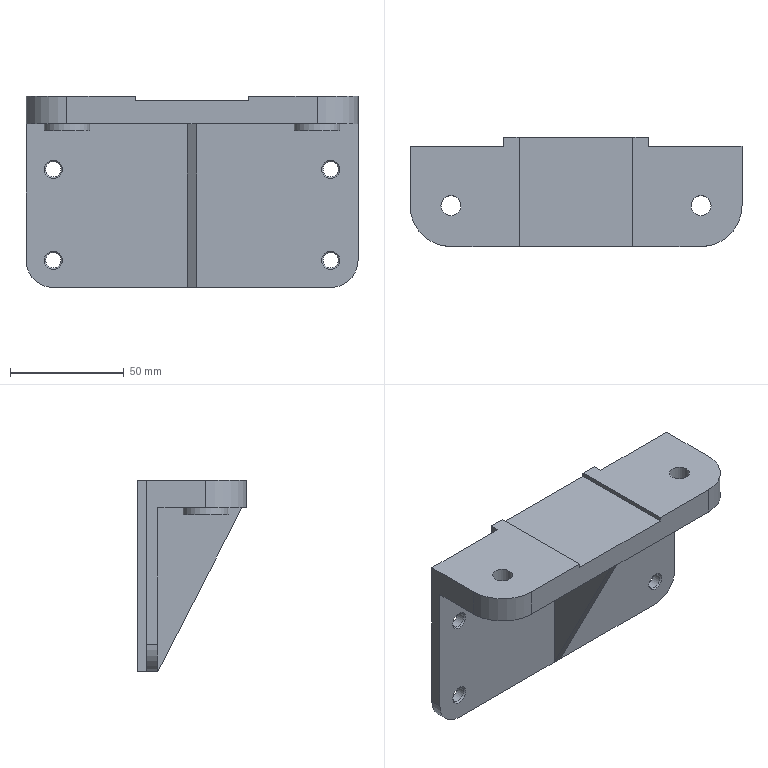Part | NX | features DATUM_CSYS 6, SIMPLE HOLE 6, SKETCH 5, SYMBOLIC_THREAD 4, EXTRUDE 3, CYLINDER 2, HOLE PACKAGE 2, BLEND 1, CPROJ 1, Intersection Curve 1, RIB 1 | 1 solid | 42 faces | box 146 x 48 x 84 mm | volume 149346 mm3 | plane 22 | cylinder 12 | cone 8 | commonest cylinder face diameters 6.8 x4 8.8 x2 20 x2 24 x2 36 x2
STEP:
#1=CARTESIAN_POINT('',(61.,37.,-16.));
#2=VERTEX_POINT('',#1);
#3=CARTESIAN_POINT('',(61.,37.,-20.));
#4=DIRECTION('',(0.,1.,0.));
#5=DIRECTION('',(0.,0.,1.));
#6=AXIS2_PLACEMENT_3D('',#3,#4,#5);
#7=CIRCLE('',#6,4.);
#8=EDGE_CURVE('',#2,#2,#7,.T.);
#9=ORIENTED_EDGE('',*,*,#8,.T.);
#10=EDGE_LOOP('',(#9));
#11=FACE_BOUND('',#10,.T.);
#12=CARTESIAN_POINT('',(61.,37.,-56.));
#13=VERTEX_POINT('',#12);
#14=CARTESIAN_POINT('',(61.,37.,-60.));
#15=DIRECTION('',(0.,1.,0.));
#16=DIRECTION('',(0.,0.,1.));
#17=AXIS2_PLACEMENT_3D('',#14,#15,#16);
#18=CIRCLE('',#17,4.);
#19=EDGE_CURVE('',#13,#13,#18,.T.);
#20=ORIENTED_EDGE('',*,*,#19,.T.);
#21=EDGE_LOOP('',(#20));
#22=FACE_BOUND('',#21,.T.);
#23=CARTESIAN_POINT('',(73.,37.,0.));
#24=VERTEX_POINT('',#23);
#25=CARTESIAN_POINT('',(2.,37.,0.));
#26=VERTEX_POINT('',#25);
#27=CARTESIAN_POINT('',(-55.,37.,0.));
#28=DIRECTION('',(-1.,0.,0.));
#29=VECTOR('',#28,1000.);
#30=LINE('',#27,#29);
#31=EDGE_CURVE('',#24,#26,#30,.T.);
#32=ORIENTED_EDGE('',*,*,#31,.T.);
#33=CARTESIAN_POINT('',(2.,37.,-72.));
#34=VERTEX_POINT('',#33);
#35=CARTESIAN_POINT('',(2.,37.,0.));
#36=DIRECTION('',(0.,0.,-1.));
#37=VECTOR('',#36,1000.);
#38=LINE('',#35,#37);
#39=EDGE_CURVE('',#26,#34,#38,.T.);
#40=ORIENTED_EDGE('',*,*,#39,.T.);
#41=CARTESIAN_POINT('',(61.,37.,-72.));
#42=VERTEX_POINT('',#41);
#43=CARTESIAN_POINT('',(73.,37.,-72.));
#44=DIRECTION('',(-1.,0.,0.));
#45=VECTOR('',#44,1000.);
#46=LINE('',#43,#45);
#47=EDGE_CURVE('',#42,#34,#46,.T.);
#48=ORIENTED_EDGE('',*,*,#47,.F.);
#49=CARTESIAN_POINT('',(73.,37.,-60.));
#50=VERTEX_POINT('',#49);
#51=CARTESIAN_POINT('',(61.,37.,-60.));
#52=DIRECTION('',(0.,1.,0.));
#53=DIRECTION('',(0.,0.,1.));
#54=AXIS2_PLACEMENT_3D('',#51,#52,#53);
#55=CIRCLE('',#54,12.);
#56=EDGE_CURVE('',#42,#50,#55,.F.);
#57=ORIENTED_EDGE('',*,*,#56,.T.);
#58=CARTESIAN_POINT('',(73.,37.,-72.));
#59=DIRECTION('',(0.,0.,1.));
#60=VECTOR('',#59,1000.);
#61=LINE('',#58,#60);
#62=EDGE_CURVE('',#50,#24,#61,.T.);
#63=ORIENTED_EDGE('',*,*,#62,.T.);
#64=EDGE_LOOP('',(#32,#40,#48,#57,#63));
#65=FACE_BOUND('',#64,.T.);
#66=CARTESIAN_POINT('',(73.,37.,-72.));
#67=DIRECTION('',(0.,1.,0.));
#68=DIRECTION('',(0.,0.,1.));
#69=AXIS2_PLACEMENT_3D('',#66,#67,#68);
#70=PLANE('',#69);
#71=ADVANCED_FACE('',(#11,#22,#65),#70,.F.);
#72=CARTESIAN_POINT('',(-50.6,16.,12.));
#73=VERTEX_POINT('',#72);
#74=CARTESIAN_POINT('',(-55.,16.,12.));
#75=DIRECTION('',(0.,0.,1.));
#76=DIRECTION('',(1.,0.,0.));
#77=AXIS2_PLACEMENT_3D('',#74,#75,#76);
#78=CIRCLE('',#77,4.4);
#79=EDGE_CURVE('',#73,#73,#78,.T.);
#80=ORIENTED_EDGE('',*,*,#79,.F.);
#81=EDGE_LOOP('',(#80));
#82=FACE_BOUND('',#81,.T.);
#83=CARTESIAN_POINT('',(-55.,-2.,12.));
#84=VERTEX_POINT('',#83);
#85=CARTESIAN_POINT('',(-25.,-2.,12.));
#86=VERTEX_POINT('',#85);
#87=CARTESIAN_POINT('',(-55.,-2.,12.));
#88=DIRECTION('',(1.,0.,0.));
#89=VECTOR('',#88,1000.);
#90=LINE('',#87,#89);
#91=EDGE_CURVE('',#84,#86,#90,.T.);
#92=ORIENTED_EDGE('',*,*,#91,.T.);
#93=CARTESIAN_POINT('',(-25.,46.,12.));
#94=VERTEX_POINT('',#93);
#95=CARTESIAN_POINT('',(-25.,-50.,12.));
#96=DIRECTION('',(0.,1.,0.));
#97=VECTOR('',#96,1000.);
#98=LINE('',#95,#97);
#99=EDGE_CURVE('',#86,#94,#98,.T.);
#100=ORIENTED_EDGE('',*,*,#99,.T.);
#101=CARTESIAN_POINT('',(-32.,46.,12.));
#102=VERTEX_POINT('',#101);
#103=CARTESIAN_POINT('',(32.,46.,12.));
#104=DIRECTION('',(-1.,0.,0.));
#105=VECTOR('',#104,1000.);
#106=LINE('',#103,#105);
#107=EDGE_CURVE('',#94,#102,#106,.T.);
#108=ORIENTED_EDGE('',*,*,#107,.T.);
#109=CARTESIAN_POINT('',(-32.,42.,12.));
#110=VERTEX_POINT('',#109);
#111=CARTESIAN_POINT('',(-32.,46.,12.));
#112=DIRECTION('',(0.,-1.,0.));
#113=VECTOR('',#112,1000.);
#114=LINE('',#111,#113);
#115=EDGE_CURVE('',#102,#110,#114,.T.);
#116=ORIENTED_EDGE('',*,*,#115,.T.);
#117=CARTESIAN_POINT('',(-73.,42.,12.));
#118=VERTEX_POINT('',#117);
#119=CARTESIAN_POINT('',(73.,42.,12.));
#120=DIRECTION('',(-1.,0.,0.));
#121=VECTOR('',#120,1000.);
#122=LINE('',#119,#121);
#123=EDGE_CURVE('',#110,#118,#122,.T.);
#124=ORIENTED_EDGE('',*,*,#123,.T.);
#125=CARTESIAN_POINT('',(-73.,16.,12.));
#126=VERTEX_POINT('',#125);
#127=CARTESIAN_POINT('',(-73.,42.,12.));
#128=DIRECTION('',(0.,-1.,0.));
#129=VECTOR('',#128,1000.);
#130=LINE('',#127,#129);
#131=EDGE_CURVE('',#118,#126,#130,.T.);
#132=ORIENTED_EDGE('',*,*,#131,.T.);
#133=CARTESIAN_POINT('',(-55.,16.,12.));
#134=DIRECTION('',(0.,0.,1.));
#135=DIRECTION('',(1.,0.,0.));
#136=AXIS2_PLACEMENT_3D('',#133,#134,#135);
#137=CIRCLE('',#136,18.);
#138=EDGE_CURVE('',#126,#84,#137,.T.);
#139=ORIENTED_EDGE('',*,*,#138,.T.);
#140=EDGE_LOOP('',(#92,#100,#108,#116,#124,#132,#139));
#141=FACE_BOUND('',#140,.T.);
#142=CARTESIAN_POINT('',(-55.,16.,12.));
#143=DIRECTION('',(0.,0.,1.));
#144=DIRECTION('',(1.,0.,0.));
#145=AXIS2_PLACEMENT_3D('',#142,#143,#144);
#146=PLANE('',#145);
#147=ADVANCED_FACE('',(#82,#141),#146,.T.);
#148=CARTESIAN_POINT('',(-61.,42.,-64.));
#149=VERTEX_POINT('',#148);
#150=CARTESIAN_POINT('',(-61.,42.,-60.));
#151=DIRECTION('',(0.,-1.,0.));
#152=DIRECTION('',(0.,0.,-1.));
#153=AXIS2_PLACEMENT_3D('',#150,#151,#152);
#154=CIRCLE('',#153,4.);
#155=EDGE_CURVE('',#149,#149,#154,.T.);
#156=ORIENTED_EDGE('',*,*,#155,.T.);
#157=EDGE_LOOP('',(#156));
#158=FACE_BOUND('',#157,.T.);
#159=CARTESIAN_POINT('',(-61.,42.,-24.));
#160=VERTEX_POINT('',#159);
#161=CARTESIAN_POINT('',(-61.,42.,-20.));
#162=DIRECTION('',(0.,-1.,0.));
#163=DIRECTION('',(0.,0.,-1.));
#164=AXIS2_PLACEMENT_3D('',#161,#162,#163);
#165=CIRCLE('',#164,4.);
#166=EDGE_CURVE('',#160,#160,#165,.T.);
#167=ORIENTED_EDGE('',*,*,#166,.T.);
#168=EDGE_LOOP('',(#167));
#169=FACE_BOUND('',#168,.T.);
#170=CARTESIAN_POINT('',(-61.,42.,-72.));
#171=VERTEX_POINT('',#170);
#172=CARTESIAN_POINT('',(-32.,42.,-72.));
#173=VERTEX_POINT('',#172);
#174=CARTESIAN_POINT('',(-73.,42.,-72.));
#175=DIRECTION('',(1.,0.,0.));
#176=VECTOR('',#175,1000.);
#177=LINE('',#174,#176);
#178=EDGE_CURVE('',#171,#173,#177,.T.);
#179=ORIENTED_EDGE('',*,*,#178,.F.);
#180=CARTESIAN_POINT('',(-73.,42.,-60.));
#181=VERTEX_POINT('',#180);
#182=CARTESIAN_POINT('',(-61.,42.,-60.));
#183=DIRECTION('',(0.,-1.,0.));
#184=DIRECTION('',(0.,0.,-1.));
#185=AXIS2_PLACEMENT_3D('',#182,#183,#184);
#186=CIRCLE('',#185,12.);
#187=EDGE_CURVE('',#171,#181,#186,.F.);
#188=ORIENTED_EDGE('',*,*,#187,.T.);
#189=CARTESIAN_POINT('',(-73.,42.,12.));
#190=DIRECTION('',(0.,0.,-1.));
#191=VECTOR('',#190,1000.);
#192=LINE('',#189,#191);
#193=EDGE_CURVE('',#118,#181,#192,.T.);
#194=ORIENTED_EDGE('',*,*,#193,.F.);
#195=ORIENTED_EDGE('',*,*,#123,.F.);
#196=CARTESIAN_POINT('',(-32.,42.,-72.));
#197=DIRECTION('',(0.,0.,1.));
#198=VECTOR('',#197,1000.);
#199=LINE('',#196,#198);
#200=EDGE_CURVE('',#173,#110,#199,.T.);
#201=ORIENTED_EDGE('',*,*,#200,.F.);
#202=EDGE_LOOP('',(#179,#188,#194,#195,#201));
#203=FACE_BOUND('',#202,.T.);
#204=CARTESIAN_POINT('',(73.,42.,12.));
#205=DIRECTION('',(0.,-1.,0.));
#206=DIRECTION('',(0.,0.,-1.));
#207=AXIS2_PLACEMENT_3D('',#204,#205,#206);
#208=PLANE('',#207);
#209=ADVANCED_FACE('',(#158,#169,#203),#208,.F.);
#210=CARTESIAN_POINT('',(-45.,16.,0.));
#211=VERTEX_POINT('',#210);
#212=CARTESIAN_POINT('',(-55.,16.,0.));
#213=DIRECTION('',(0.,0.,-1.));
#214=DIRECTION('',(1.,0.,0.));
#215=AXIS2_PLACEMENT_3D('',#212,#213,#214);
#216=CIRCLE('',#215,10.);
#217=EDGE_CURVE('',#211,#211,#216,.T.);
#218=ORIENTED_EDGE('',*,*,#217,.F.);
#219=EDGE_LOOP('',(#218));
#220=FACE_BOUND('',#219,.T.);
#221=CARTESIAN_POINT('',(65.,16.,0.));
#222=VERTEX_POINT('',#221);
#223=CARTESIAN_POINT('',(55.,16.,0.));
#224=DIRECTION('',(0.,0.,-1.));
#225=DIRECTION('',(1.,0.,0.));
#226=AXIS2_PLACEMENT_3D('',#223,#224,#225);
#227=CIRCLE('',#226,10.);
#228=EDGE_CURVE('',#222,#222,#227,.T.);
#229=ORIENTED_EDGE('',*,*,#228,.F.);
#230=EDGE_LOOP('',(#229));
#231=FACE_BOUND('',#230,.T.);
#232=CARTESIAN_POINT('',(-2.,0.,0.));
#233=VERTEX_POINT('',#232);
#234=CARTESIAN_POINT('',(2.,0.,0.));
#235=VERTEX_POINT('',#234);
#236=CARTESIAN_POINT('',(2.,0.,0.));
#237=DIRECTION('',(-1.,0.,0.));
#238=VECTOR('',#237,1000.);
#239=LINE('',#236,#238);
#240=EDGE_CURVE('',#233,#235,#239,.F.);
#241=ORIENTED_EDGE('',*,*,#240,.T.);
#242=CARTESIAN_POINT('',(2.,0.,0.));
#243=DIRECTION('',(0.,1.,0.));
#244=VECTOR('',#243,1000.);
#245=LINE('',#242,#244);
#246=EDGE_CURVE('',#235,#26,#245,.T.);
#247=ORIENTED_EDGE('',*,*,#246,.T.);
#248=ORIENTED_EDGE('',*,*,#31,.F.);
#249=CARTESIAN_POINT('',(73.,16.,0.));
#250=VERTEX_POINT('',#249);
#251=CARTESIAN_POINT('',(73.,16.,0.));
#252=DIRECTION('',(0.,1.,0.));
#253=VECTOR('',#252,1000.);
#254=LINE('',#251,#253);
#255=EDGE_CURVE('',#250,#24,#254,.T.);
#256=ORIENTED_EDGE('',*,*,#255,.F.);
#257=CARTESIAN_POINT('',(55.,-2.,0.));
#258=VERTEX_POINT('',#257);
#259=CARTESIAN_POINT('',(55.,16.,0.));
#260=DIRECTION('',(0.,0.,1.));
#261=DIRECTION('',(1.,0.,0.));
#262=AXIS2_PLACEMENT_3D('',#259,#260,#261);
#263=CIRCLE('',#262,18.);
#264=EDGE_CURVE('',#258,#250,#263,.T.);
#265=ORIENTED_EDGE('',*,*,#264,.F.);
#266=CARTESIAN_POINT('',(-55.,-2.,0.));
#267=VERTEX_POINT('',#266);
#268=CARTESIAN_POINT('',(-55.,-2.,0.));
#269=DIRECTION('',(1.,0.,0.));
#270=VECTOR('',#269,1000.);
#271=LINE('',#268,#270);
#272=EDGE_CURVE('',#267,#258,#271,.T.);
#273=ORIENTED_EDGE('',*,*,#272,.F.);
#274=CARTESIAN_POINT('',(-73.,16.,0.));
#275=VERTEX_POINT('',#274);
#276=CARTESIAN_POINT('',(-55.,16.,0.));
#277=DIRECTION('',(0.,0.,1.));
#278=DIRECTION('',(1.,0.,0.));
#279=AXIS2_PLACEMENT_3D('',#276,#277,#278);
#280=CIRCLE('',#279,18.);
#281=EDGE_CURVE('',#275,#267,#280,.T.);
#282=ORIENTED_EDGE('',*,*,#281,.F.);
#283=CARTESIAN_POINT('',(-73.,37.,0.));
#284=VERTEX_POINT('',#283);
#285=CARTESIAN_POINT('',(-73.,42.,0.));
#286=DIRECTION('',(0.,-1.,0.));
#287=VECTOR('',#286,1000.);
#288=LINE('',#285,#287);
#289=EDGE_CURVE('',#284,#275,#288,.T.);
#290=ORIENTED_EDGE('',*,*,#289,.F.);
#291=CARTESIAN_POINT('',(-2.,37.,0.));
#292=VERTEX_POINT('',#291);
#293=CARTESIAN_POINT('',(-55.,37.,0.));
#294=DIRECTION('',(-1.,0.,0.));
#295=VECTOR('',#294,1000.);
#296=LINE('',#293,#295);
#297=EDGE_CURVE('',#292,#284,#296,.T.);
#298=ORIENTED_EDGE('',*,*,#297,.F.);
#299=CARTESIAN_POINT('',(-2.,0.,0.));
#300=DIRECTION('',(0.,1.,0.));
#301=VECTOR('',#300,1000.);
#302=LINE('',#299,#301);
#303=EDGE_CURVE('',#292,#233,#302,.F.);
#304=ORIENTED_EDGE('',*,*,#303,.T.);
#305=EDGE_LOOP('',(#241,#247,#248,#256,#265,#273,#282,#290,#298,#304));
#306=FACE_BOUND('',#305,.T.);
#307=CARTESIAN_POINT('',(-55.,16.,0.));
#308=DIRECTION('',(0.,0.,1.));
#309=DIRECTION('',(1.,0.,0.));
#310=AXIS2_PLACEMENT_3D('',#307,#308,#309);
#311=PLANE('',#310);
#312=ADVANCED_FACE('',(#220,#231,#306),#311,.F.);
#313=ORIENTED_EDGE('',*,*,#193,.T.);
#314=CARTESIAN_POINT('',(-73.,37.,-60.));
#315=VERTEX_POINT('',#314);
#316=CARTESIAN_POINT('',(-73.,37.,-60.));
#317=DIRECTION('',(0.,1.,0.));
#318=VECTOR('',#317,1000.);
#319=LINE('',#316,#318);
#320=EDGE_CURVE('',#181,#315,#319,.F.);
#321=ORIENTED_EDGE('',*,*,#320,.T.);
#322=CARTESIAN_POINT('',(-73.,37.,-72.));
#323=DIRECTION('',(0.,0.,1.));
#324=VECTOR('',#323,1000.);
#325=LINE('',#322,#324);
#326=EDGE_CURVE('',#315,#284,#325,.T.);
#327=ORIENTED_EDGE('',*,*,#326,.T.);
#328=ORIENTED_EDGE('',*,*,#289,.T.);
#329=CARTESIAN_POINT('',(-73.,16.,12.));
#330=DIRECTION('',(0.,0.,-1.));
#331=VECTOR('',#330,1000.);
#332=LINE('',#329,#331);
#333=EDGE_CURVE('',#126,#275,#332,.T.);
#334=ORIENTED_EDGE('',*,*,#333,.F.);
#335=ORIENTED_EDGE('',*,*,#131,.F.);
#336=EDGE_LOOP('',(#313,#321,#327,#328,#334,#335));
#337=FACE_BOUND('',#336,.T.);
#338=CARTESIAN_POINT('',(-73.,42.,12.));
#339=DIRECTION('',(1.,0.,0.));
#340=DIRECTION('',(0.,0.,-1.));
#341=AXIS2_PLACEMENT_3D('',#338,#339,#340);
#342=PLANE('',#341);
#343=ADVANCED_FACE('',(#337),#342,.F.);
#344=ORIENTED_EDGE('',*,*,#281,.T.);
#345=CARTESIAN_POINT('',(-55.,-2.,12.));
#346=DIRECTION('',(0.,0.,-1.));
#347=VECTOR('',#346,1000.);
#348=LINE('',#345,#347);
#349=EDGE_CURVE('',#84,#267,#348,.T.);
#350=ORIENTED_EDGE('',*,*,#349,.F.);
#351=ORIENTED_EDGE('',*,*,#138,.F.);
#352=ORIENTED_EDGE('',*,*,#333,.T.);
#353=EDGE_LOOP('',(#344,#350,#351,#352));
#354=FACE_BOUND('',#353,.T.);
#355=CARTESIAN_POINT('',(-55.,16.,12.));
#356=DIRECTION('',(0.,0.,-1.));
#357=DIRECTION('',(-1.,0.,0.));
#358=AXIS2_PLACEMENT_3D('',#355,#356,#357);
#359=CYLINDRICAL_SURFACE('',#358,18.);
#360=ADVANCED_FACE('',(#354),#359,.T.);
#361=CARTESIAN_POINT('',(25.,-2.,10.143));
#362=VERTEX_POINT('',#361);
#363=CARTESIAN_POINT('',(-25.,-2.,10.143));
#364=VERTEX_POINT('',#363);
#365=CARTESIAN_POINT('',(-55.,-2.,10.143));
#366=DIRECTION('',(-1.,0.,0.));
#367=VECTOR('',#366,1000.);
#368=LINE('',#365,#367);
#369=EDGE_CURVE('',#362,#364,#368,.T.);
#370=ORIENTED_EDGE('',*,*,#369,.T.);
#371=CARTESIAN_POINT('',(-25.,-2.,12.));
#372=DIRECTION('',(0.,0.,1.));
#373=VECTOR('',#372,1000.);
#374=LINE('',#371,#373);
#375=EDGE_CURVE('',#364,#86,#374,.T.);
#376=ORIENTED_EDGE('',*,*,#375,.T.);
#377=ORIENTED_EDGE('',*,*,#91,.F.);
#378=ORIENTED_EDGE('',*,*,#349,.T.);
#379=ORIENTED_EDGE('',*,*,#272,.T.);
#380=CARTESIAN_POINT('',(55.,-2.,12.));
#381=VERTEX_POINT('',#380);
#382=CARTESIAN_POINT('',(55.,-2.,12.));
#383=DIRECTION('',(0.,0.,-1.));
#384=VECTOR('',#383,1000.);
#385=LINE('',#382,#384);
#386=EDGE_CURVE('',#381,#258,#385,.T.);
#387=ORIENTED_EDGE('',*,*,#386,.F.);
#388=CARTESIAN_POINT('',(25.,-2.,12.));
#389=VERTEX_POINT('',#388);
#390=CARTESIAN_POINT('',(-55.,-2.,12.));
#391=DIRECTION('',(1.,0.,0.));
#392=VECTOR('',#391,1000.);
#393=LINE('',#390,#392);
#394=EDGE_CURVE('',#389,#381,#393,.T.);
#395=ORIENTED_EDGE('',*,*,#394,.F.);
#396=CARTESIAN_POINT('',(25.,-2.,12.));
#397=DIRECTION('',(0.,0.,-1.));
#398=VECTOR('',#397,1000.);
#399=LINE('',#396,#398);
#400=EDGE_CURVE('',#389,#362,#399,.T.);
#401=ORIENTED_EDGE('',*,*,#400,.T.);
#402=EDGE_LOOP('',(#370,#376,#377,#378,#379,#387,#395,#401));
#403=FACE_BOUND('',#402,.T.);
#404=CARTESIAN_POINT('',(-55.,-2.,12.));
#405=DIRECTION('',(0.,1.,0.));
#406=DIRECTION('',(-1.,0.,0.));
#407=AXIS2_PLACEMENT_3D('',#404,#405,#406);
#408=PLANE('',#407);
#409=ADVANCED_FACE('',(#403),#408,.F.);
#410=ORIENTED_EDGE('',*,*,#264,.T.);
#411=CARTESIAN_POINT('',(73.,16.,12.));
#412=VERTEX_POINT('',#411);
#413=CARTESIAN_POINT('',(73.,16.,12.));
#414=DIRECTION('',(0.,0.,-1.));
#415=VECTOR('',#414,1000.);
#416=LINE('',#413,#415);
#417=EDGE_CURVE('',#412,#250,#416,.T.);
#418=ORIENTED_EDGE('',*,*,#417,.F.);
#419=CARTESIAN_POINT('',(55.,16.,12.));
#420=DIRECTION('',(0.,0.,1.));
#421=DIRECTION('',(1.,0.,0.));
#422=AXIS2_PLACEMENT_3D('',#419,#420,#421);
#423=CIRCLE('',#422,18.);
#424=EDGE_CURVE('',#381,#412,#423,.T.);
#425=ORIENTED_EDGE('',*,*,#424,.F.);
#426=ORIENTED_EDGE('',*,*,#386,.T.);
#427=EDGE_LOOP('',(#410,#418,#425,#426));
#428=FACE_BOUND('',#427,.T.);
#429=CARTESIAN_POINT('',(55.,16.,12.));
#430=DIRECTION('',(0.,0.,-1.));
#431=DIRECTION('',(-1.,0.,0.));
#432=AXIS2_PLACEMENT_3D('',#429,#430,#431);
#433=CYLINDRICAL_SURFACE('',#432,18.);
#434=ADVANCED_FACE('',(#428),#433,.T.);
#435=ORIENTED_EDGE('',*,*,#62,.F.);
#436=CARTESIAN_POINT('',(73.,42.,-60.));
#437=VERTEX_POINT('',#436);
#438=CARTESIAN_POINT('',(73.,42.,-60.));
#439=DIRECTION('',(0.,-1.,0.));
#440=VECTOR('',#439,1000.);
#441=LINE('',#438,#440);
#442=EDGE_CURVE('',#50,#437,#441,.F.);
#443=ORIENTED_EDGE('',*,*,#442,.T.);
#444=CARTESIAN_POINT('',(73.,42.,12.));
#445=VERTEX_POINT('',#444);
#446=CARTESIAN_POINT('',(73.,42.,12.));
#447=DIRECTION('',(0.,0.,-1.));
#448=VECTOR('',#447,1000.);
#449=LINE('',#446,#448);
#450=EDGE_CURVE('',#445,#437,#449,.T.);
#451=ORIENTED_EDGE('',*,*,#450,.F.);
#452=CARTESIAN_POINT('',(73.,16.,12.));
#453=DIRECTION('',(0.,1.,0.));
#454=VECTOR('',#453,1000.);
#455=LINE('',#452,#454);
#456=EDGE_CURVE('',#412,#445,#455,.T.);
#457=ORIENTED_EDGE('',*,*,#456,.F.);
#458=ORIENTED_EDGE('',*,*,#417,.T.);
#459=ORIENTED_EDGE('',*,*,#255,.T.);
#460=EDGE_LOOP('',(#435,#443,#451,#457,#458,#459));
#461=FACE_BOUND('',#460,.T.);
#462=CARTESIAN_POINT('',(73.,16.,12.));
#463=DIRECTION('',(-1.,0.,0.));
#464=DIRECTION('',(0.,-1.,0.));
#465=AXIS2_PLACEMENT_3D('',#462,#463,#464);
#466=PLANE('',#465);
#467=ADVANCED_FACE('',(#461),#466,.F.);
#468=CARTESIAN_POINT('',(61.,42.,-64.));
#469=VERTEX_POINT('',#468);
#470=CARTESIAN_POINT('',(61.,42.,-60.));
#471=DIRECTION('',(0.,-1.,0.));
#472=DIRECTION('',(0.,0.,-1.));
#473=AXIS2_PLACEMENT_3D('',#470,#471,#472);
#474=CIRCLE('',#473,4.);
#475=EDGE_CURVE('',#469,#469,#474,.T.);
#476=ORIENTED_EDGE('',*,*,#475,.T.);
#477=EDGE_LOOP('',(#476));
#478=FACE_BOUND('',#477,.T.);
#479=CARTESIAN_POINT('',(61.,42.,-24.));
#480=VERTEX_POINT('',#479);
#481=CARTESIAN_POINT('',(61.,42.,-20.));
#482=DIRECTION('',(0.,-1.,0.));
#483=DIRECTION('',(0.,0.,-1.));
#484=AXIS2_PLACEMENT_3D('',#481,#482,#483);
#485=CIRCLE('',#484,4.);
#486=EDGE_CURVE('',#480,#480,#485,.T.);
#487=ORIENTED_EDGE('',*,*,#486,.T.);
#488=EDGE_LOOP('',(#487));
#489=FACE_BOUND('',#488,.T.);
#490=ORIENTED_EDGE('',*,*,#450,.T.);
#491=CARTESIAN_POINT('',(61.,42.,-72.));
#492=VERTEX_POINT('',#491);
#493=CARTESIAN_POINT('',(61.,42.,-60.));
#494=DIRECTION('',(0.,-1.,0.));
#495=DIRECTION('',(0.,0.,-1.));
#496=AXIS2_PLACEMENT_3D('',#493,#494,#495);
#497=CIRCLE('',#496,12.);
#498=EDGE_CURVE('',#437,#492,#497,.F.);
#499=ORIENTED_EDGE('',*,*,#498,.T.);
#500=CARTESIAN_POINT('',(32.,42.,-72.));
#501=VERTEX_POINT('',#500);
#502=CARTESIAN_POINT('',(-73.,42.,-72.));
#503=DIRECTION('',(1.,0.,0.));
#504=VECTOR('',#503,1000.);
#505=LINE('',#502,#504);
#506=EDGE_CURVE('',#501,#492,#505,.T.);
#507=ORIENTED_EDGE('',*,*,#506,.F.);
#508=CARTESIAN_POINT('',(32.,42.,12.));
#509=VERTEX_POINT('',#508);
#510=CARTESIAN_POINT('',(32.,42.,-72.));
#511=DIRECTION('',(0.,0.,1.));
#512=VECTOR('',#511,1000.);
#513=LINE('',#510,#512);
#514=EDGE_CURVE('',#501,#509,#513,.T.);
#515=ORIENTED_EDGE('',*,*,#514,.T.);
#516=CARTESIAN_POINT('',(73.,42.,12.));
#517=DIRECTION('',(-1.,0.,0.));
#518=VECTOR('',#517,1000.);
#519=LINE('',#516,#518);
#520=EDGE_CURVE('',#445,#509,#519,.T.);
#521=ORIENTED_EDGE('',*,*,#520,.F.);
#522=EDGE_LOOP('',(#490,#499,#507,#515,#521));
#523=FACE_BOUND('',#522,.T.);
#524=CARTESIAN_POINT('',(73.,42.,12.));
#525=DIRECTION('',(0.,-1.,0.));
#526=DIRECTION('',(0.,0.,-1.));
#527=AXIS2_PLACEMENT_3D('',#524,#525,#526);
#528=PLANE('',#527);
#529=ADVANCED_FACE('',(#478,#489,#523),#528,.F.);
#530=CARTESIAN_POINT('',(59.4,16.,12.));
#531=VERTEX_POINT('',#530);
#532=CARTESIAN_POINT('',(55.,16.,12.));
#533=DIRECTION('',(0.,0.,1.));
#534=DIRECTION('',(1.,0.,0.));
#535=AXIS2_PLACEMENT_3D('',#532,#533,#534);
#536=CIRCLE('',#535,4.4);
#537=EDGE_CURVE('',#531,#531,#536,.T.);
#538=ORIENTED_EDGE('',*,*,#537,.F.);
#539=EDGE_LOOP('',(#538));
#540=FACE_BOUND('',#539,.T.);
#541=CARTESIAN_POINT('',(25.,46.,12.));
#542=VERTEX_POINT('',#541);
#543=CARTESIAN_POINT('',(25.,-50.,12.));
#544=DIRECTION('',(0.,1.,0.));
#545=VECTOR('',#544,1000.);
#546=LINE('',#543,#545);
#547=EDGE_CURVE('',#389,#542,#546,.T.);
#548=ORIENTED_EDGE('',*,*,#547,.F.);
#549=ORIENTED_EDGE('',*,*,#394,.T.);
#550=ORIENTED_EDGE('',*,*,#424,.T.);
#551=ORIENTED_EDGE('',*,*,#456,.T.);
#552=ORIENTED_EDGE('',*,*,#520,.T.);
#553=CARTESIAN_POINT('',(32.,46.,12.));
#554=VERTEX_POINT('',#553);
#555=CARTESIAN_POINT('',(32.,42.,12.));
#556=DIRECTION('',(0.,1.,0.));
#557=VECTOR('',#556,1000.);
#558=LINE('',#555,#557);
#559=EDGE_CURVE('',#509,#554,#558,.T.);
#560=ORIENTED_EDGE('',*,*,#559,.T.);
#561=CARTESIAN_POINT('',(32.,46.,12.));
#562=DIRECTION('',(-1.,0.,0.));
#563=VECTOR('',#562,1000.);
#564=LINE('',#561,#563);
#565=EDGE_CURVE('',#554,#542,#564,.T.);
#566=ORIENTED_EDGE('',*,*,#565,.T.);
#567=EDGE_LOOP('',(#548,#549,#550,#551,#552,#560,#566));
#568=FACE_BOUND('',#567,.T.);
#569=CARTESIAN_POINT('',(-55.,16.,12.));
#570=DIRECTION('',(0.,0.,1.));
#571=DIRECTION('',(1.,0.,0.));
#572=AXIS2_PLACEMENT_3D('',#569,#570,#571);
#573=PLANE('',#572);
#574=ADVANCED_FACE('',(#540,#568),#573,.T.);
#575=CARTESIAN_POINT('',(-61.,37.,-56.));
#576=VERTEX_POINT('',#575);
#577=CARTESIAN_POINT('',(-61.,37.,-60.));
#578=DIRECTION('',(0.,1.,0.));
#579=DIRECTION('',(0.,0.,1.));
#580=AXIS2_PLACEMENT_3D('',#577,#578,#579);
#581=CIRCLE('',#580,4.);
#582=EDGE_CURVE('',#576,#576,#581,.T.);
#583=ORIENTED_EDGE('',*,*,#582,.T.);
#584=EDGE_LOOP('',(#583));
#585=FACE_BOUND('',#584,.T.);
#586=CARTESIAN_POINT('',(-61.,37.,-16.));
#587=VERTEX_POINT('',#586);
#588=CARTESIAN_POINT('',(-61.,37.,-20.));
#589=DIRECTION('',(0.,1.,0.));
#590=DIRECTION('',(0.,0.,1.));
#591=AXIS2_PLACEMENT_3D('',#588,#589,#590);
#592=CIRCLE('',#591,4.);
#593=EDGE_CURVE('',#587,#587,#592,.T.);
#594=ORIENTED_EDGE('',*,*,#593,.T.);
#595=EDGE_LOOP('',(#594));
#596=FACE_BOUND('',#595,.T.);
#597=CARTESIAN_POINT('',(-2.,37.,-72.));
#598=VERTEX_POINT('',#597);
#599=CARTESIAN_POINT('',(-61.,37.,-72.));
#600=VERTEX_POINT('',#599);
#601=CARTESIAN_POINT('',(73.,37.,-72.));
#602=DIRECTION('',(-1.,0.,0.));
#603=VECTOR('',#602,1000.);
#604=LINE('',#601,#603);
#605=EDGE_CURVE('',#598,#600,#604,.T.);
#606=ORIENTED_EDGE('',*,*,#605,.F.);
#607=CARTESIAN_POINT('',(-2.,37.,0.));
#608=DIRECTION('',(0.,0.,-1.));
#609=VECTOR('',#608,1000.);
#610=LINE('',#607,#609);
#611=EDGE_CURVE('',#598,#292,#610,.F.);
#612=ORIENTED_EDGE('',*,*,#611,.T.);
#613=ORIENTED_EDGE('',*,*,#297,.T.);
#614=ORIENTED_EDGE('',*,*,#326,.F.);
#615=CARTESIAN_POINT('',(-61.,37.,-60.));
#616=DIRECTION('',(0.,1.,0.));
#617=DIRECTION('',(0.,0.,1.));
#618=AXIS2_PLACEMENT_3D('',#615,#616,#617);
#619=CIRCLE('',#618,12.);
#620=EDGE_CURVE('',#315,#600,#619,.F.);
#621=ORIENTED_EDGE('',*,*,#620,.T.);
#622=EDGE_LOOP('',(#606,#612,#613,#614,#621));
#623=FACE_BOUND('',#622,.T.);
#624=CARTESIAN_POINT('',(73.,37.,-72.));
#625=DIRECTION('',(0.,1.,0.));
#626=DIRECTION('',(0.,0.,1.));
#627=AXIS2_PLACEMENT_3D('',#624,#625,#626);
#628=PLANE('',#627);
#629=ADVANCED_FACE('',(#585,#596,#623),#628,.F.);
#630=ORIENTED_EDGE('',*,*,#47,.T.);
#631=CARTESIAN_POINT('',(2.,37.,-72.));
#632=DIRECTION('',(-1.,0.,0.));
#633=VECTOR('',#632,1000.);
#634=LINE('',#631,#633);
#635=EDGE_CURVE('',#34,#598,#634,.T.);
#636=ORIENTED_EDGE('',*,*,#635,.T.);
#637=ORIENTED_EDGE('',*,*,#605,.T.);
#638=CARTESIAN_POINT('',(-61.,42.,-72.));
#639=DIRECTION('',(0.,1.,0.));
#640=VECTOR('',#639,1000.);
#641=LINE('',#638,#640);
#642=EDGE_CURVE('',#600,#171,#641,.T.);
#643=ORIENTED_EDGE('',*,*,#642,.T.);
#644=ORIENTED_EDGE('',*,*,#178,.T.);
#645=CARTESIAN_POINT('',(-32.,46.,-72.));
#646=VERTEX_POINT('',#645);
#647=CARTESIAN_POINT('',(-32.,46.,-72.));
#648=DIRECTION('',(0.,-1.,0.));
#649=VECTOR('',#648,1000.);
#650=LINE('',#647,#649);
#651=EDGE_CURVE('',#646,#173,#650,.T.);
#652=ORIENTED_EDGE('',*,*,#651,.F.);
#653=CARTESIAN_POINT('',(32.,46.,-72.));
#654=VERTEX_POINT('',#653);
#655=CARTESIAN_POINT('',(32.,46.,-72.));
#656=DIRECTION('',(-1.,0.,0.));
#657=VECTOR('',#656,1000.);
#658=LINE('',#655,#657);
#659=EDGE_CURVE('',#654,#646,#658,.T.);
#660=ORIENTED_EDGE('',*,*,#659,.F.);
#661=CARTESIAN_POINT('',(32.,42.,-72.));
#662=DIRECTION('',(0.,1.,0.));
#663=VECTOR('',#662,1000.);
#664=LINE('',#661,#663);
#665=EDGE_CURVE('',#501,#654,#664,.T.);
#666=ORIENTED_EDGE('',*,*,#665,.F.);
#667=ORIENTED_EDGE('',*,*,#506,.T.);
#668=CARTESIAN_POINT('',(61.,37.,-72.));
#669=DIRECTION('',(0.,-1.,0.));
#670=VECTOR('',#669,1000.);
#671=LINE('',#668,#670);
#672=EDGE_CURVE('',#492,#42,#671,.T.);
#673=ORIENTED_EDGE('',*,*,#672,.T.);
#674=EDGE_LOOP('',(#630,#636,#637,#643,#644,#652,#660,#666,#667,#673));
#675=FACE_BOUND('',#674,.T.);
#676=CARTESIAN_POINT('',(0.,0.,-72.));
#677=DIRECTION('',(0.,0.,-1.));
#678=DIRECTION('',(-1.,0.,0.));
#679=AXIS2_PLACEMENT_3D('',#676,#677,#678);
#680=PLANE('',#679);
#681=ADVANCED_FACE('',(#675),#680,.T.);
#682=ORIENTED_EDGE('',*,*,#115,.F.);
#683=CARTESIAN_POINT('',(-32.,46.,-72.));
#684=DIRECTION('',(0.,0.,1.));
#685=VECTOR('',#684,1000.);
#686=LINE('',#683,#685);
#687=EDGE_CURVE('',#646,#102,#686,.T.);
#688=ORIENTED_EDGE('',*,*,#687,.F.);
#689=ORIENTED_EDGE('',*,*,#651,.T.);
#690=ORIENTED_EDGE('',*,*,#200,.T.);
#691=EDGE_LOOP('',(#682,#688,#689,#690));
#692=FACE_BOUND('',#691,.T.);
#693=CARTESIAN_POINT('',(-32.,46.,-72.));
#694=DIRECTION('',(-1.,0.,0.));
#695=DIRECTION('',(0.,0.,1.));
#696=AXIS2_PLACEMENT_3D('',#693,#694,#695);
#697=PLANE('',#696);
#698=ADVANCED_FACE('',(#692),#697,.T.);
#699=ORIENTED_EDGE('',*,*,#559,.F.);
#700=ORIENTED_EDGE('',*,*,#514,.F.);
#701=ORIENTED_EDGE('',*,*,#665,.T.);
#702=CARTESIAN_POINT('',(32.,46.,-72.));
#703=DIRECTION('',(0.,0.,1.));
#704=VECTOR('',#703,1000.);
#705=LINE('',#702,#704);
#706=EDGE_CURVE('',#654,#554,#705,.T.);
#707=ORIENTED_EDGE('',*,*,#706,.T.);
#708=EDGE_LOOP('',(#699,#700,#701,#707));
#709=FACE_BOUND('',#708,.T.);
#710=CARTESIAN_POINT('',(32.,42.,-72.));
#711=DIRECTION('',(1.,0.,0.));
#712=DIRECTION('',(0.,0.,-1.));
#713=AXIS2_PLACEMENT_3D('',#710,#711,#712);
#714=PLANE('',#713);
#715=ADVANCED_FACE('',(#709),#714,.T.);
#716=CARTESIAN_POINT('',(-25.,46.,10.143));
#717=VERTEX_POINT('',#716);
#718=CARTESIAN_POINT('',(-25.,46.,10.143));
#719=DIRECTION('',(0.,0.,1.));
#720=VECTOR('',#719,1000.);
#721=LINE('',#718,#720);
#722=EDGE_CURVE('',#717,#94,#721,.T.);
#723=ORIENTED_EDGE('',*,*,#722,.F.);
#724=CARTESIAN_POINT('',(25.,46.,10.143));
#725=VERTEX_POINT('',#724);
#726=CARTESIAN_POINT('',(25.,46.,10.143));
#727=DIRECTION('',(-1.,0.,0.));
#728=VECTOR('',#727,1000.);
#729=LINE('',#726,#728);
#730=EDGE_CURVE('',#725,#717,#729,.T.);
#731=ORIENTED_EDGE('',*,*,#730,.F.);
#732=CARTESIAN_POINT('',(25.,46.,12.));
#733=DIRECTION('',(0.,0.,-1.));
#734=VECTOR('',#733,1000.);
#735=LINE('',#732,#734);
#736=EDGE_CURVE('',#542,#725,#735,.T.);
#737=ORIENTED_EDGE('',*,*,#736,.F.);
#738=ORIENTED_EDGE('',*,*,#565,.F.);
#739=ORIENTED_EDGE('',*,*,#706,.F.);
#740=ORIENTED_EDGE('',*,*,#659,.T.);
#741=ORIENTED_EDGE('',*,*,#687,.T.);
#742=ORIENTED_EDGE('',*,*,#107,.F.);
#743=EDGE_LOOP('',(#723,#731,#737,#738,#739,#740,#741,#742));
#744=FACE_BOUND('',#743,.T.);
#745=CARTESIAN_POINT('',(32.,46.,-72.));
#746=DIRECTION('',(0.,1.,0.));
#747=DIRECTION('',(0.,0.,1.));
#748=AXIS2_PLACEMENT_3D('',#745,#746,#747);
#749=PLANE('',#748);
#750=ADVANCED_FACE('',(#744),#749,.T.);
#751=CARTESIAN_POINT('',(-25.,-50.,10.143));
#752=DIRECTION('',(0.,1.,0.));
#753=VECTOR('',#752,1000.);
#754=LINE('',#751,#753);
#755=EDGE_CURVE('',#717,#364,#754,.F.);
#756=ORIENTED_EDGE('',*,*,#755,.F.);
#757=ORIENTED_EDGE('',*,*,#722,.T.);
#758=ORIENTED_EDGE('',*,*,#99,.F.);
#759=ORIENTED_EDGE('',*,*,#375,.F.);
#760=EDGE_LOOP('',(#756,#757,#758,#759));
#761=FACE_BOUND('',#760,.T.);
#762=CARTESIAN_POINT('',(-25.,-50.,10.143));
#763=DIRECTION('',(-1.,0.,0.));
#764=DIRECTION('',(0.,0.,1.));
#765=AXIS2_PLACEMENT_3D('',#762,#763,#764);
#766=PLANE('',#765);
#767=ADVANCED_FACE('',(#761),#766,.F.);
#768=ORIENTED_EDGE('',*,*,#547,.T.);
#769=ORIENTED_EDGE('',*,*,#736,.T.);
#770=CARTESIAN_POINT('',(25.,-50.,10.143));
#771=DIRECTION('',(0.,1.,0.));
#772=VECTOR('',#771,1000.);
#773=LINE('',#770,#772);
#774=EDGE_CURVE('',#725,#362,#773,.F.);
#775=ORIENTED_EDGE('',*,*,#774,.T.);
#776=ORIENTED_EDGE('',*,*,#400,.F.);
#777=EDGE_LOOP('',(#768,#769,#775,#776));
#778=FACE_BOUND('',#777,.T.);
#779=CARTESIAN_POINT('',(25.,-50.,12.));
#780=DIRECTION('',(1.,0.,0.));
#781=DIRECTION('',(0.,0.,-1.));
#782=AXIS2_PLACEMENT_3D('',#779,#780,#781);
#783=PLANE('',#782);
#784=ADVANCED_FACE('',(#778),#783,.F.);
#785=ORIENTED_EDGE('',*,*,#774,.F.);
#786=ORIENTED_EDGE('',*,*,#730,.T.);
#787=ORIENTED_EDGE('',*,*,#755,.T.);
#788=ORIENTED_EDGE('',*,*,#369,.F.);
#789=EDGE_LOOP('',(#785,#786,#787,#788));
#790=FACE_BOUND('',#789,.T.);
#791=CARTESIAN_POINT('',(25.,-50.,10.143));
#792=DIRECTION('',(0.,0.,-1.));
#793=DIRECTION('',(-1.,0.,0.));
#794=AXIS2_PLACEMENT_3D('',#791,#792,#793);
#795=PLANE('',#794);
#796=ADVANCED_FACE('',(#790),#795,.F.);
#797=ORIENTED_EDGE('',*,*,#620,.F.);
#798=ORIENTED_EDGE('',*,*,#320,.F.);
#799=ORIENTED_EDGE('',*,*,#187,.F.);
#800=ORIENTED_EDGE('',*,*,#642,.F.);
#801=EDGE_LOOP('',(#797,#798,#799,#800));
#802=FACE_BOUND('',#801,.T.);
#803=CARTESIAN_POINT('',(-61.,0.,-60.));
#804=DIRECTION('',(0.,-1.,0.));
#805=DIRECTION('',(0.,0.,-1.));
#806=AXIS2_PLACEMENT_3D('',#803,#804,#805);
#807=CYLINDRICAL_SURFACE('',#806,12.);
#808=ADVANCED_FACE('',(#802),#807,.T.);
#809=ORIENTED_EDGE('',*,*,#498,.F.);
#810=ORIENTED_EDGE('',*,*,#442,.F.);
#811=ORIENTED_EDGE('',*,*,#56,.F.);
#812=ORIENTED_EDGE('',*,*,#672,.F.);
#813=EDGE_LOOP('',(#809,#810,#811,#812));
#814=FACE_BOUND('',#813,.T.);
#815=CARTESIAN_POINT('',(61.,0.,-60.));
#816=DIRECTION('',(0.,1.,0.));
#817=DIRECTION('',(-1.,0.,0.));
#818=AXIS2_PLACEMENT_3D('',#815,#816,#817);
#819=CYLINDRICAL_SURFACE('',#818,12.);
#820=ADVANCED_FACE('',(#814),#819,.T.);
#821=CARTESIAN_POINT('',(59.4,16.,-3.));
#822=VERTEX_POINT('',#821);
#823=CARTESIAN_POINT('',(55.,16.,-3.));
#824=DIRECTION('',(0.,0.,1.));
#825=DIRECTION('',(1.,0.,0.));
#826=AXIS2_PLACEMENT_3D('',#823,#824,#825);
#827=CIRCLE('',#826,4.4);
#828=EDGE_CURVE('',#822,#822,#827,.T.);
#829=ORIENTED_EDGE('',*,*,#828,.T.);
#830=EDGE_LOOP('',(#829));
#831=FACE_BOUND('',#830,.T.);
#832=CARTESIAN_POINT('',(65.,16.,-3.));
#833=VERTEX_POINT('',#832);
#834=CARTESIAN_POINT('',(55.,16.,-3.));
#835=DIRECTION('',(0.,0.,1.));
#836=DIRECTION('',(1.,0.,0.));
#837=AXIS2_PLACEMENT_3D('',#834,#835,#836);
#838=CIRCLE('',#837,10.);
#839=EDGE_CURVE('',#833,#833,#838,.T.);
#840=ORIENTED_EDGE('',*,*,#839,.F.);
#841=EDGE_LOOP('',(#840));
#842=FACE_BOUND('',#841,.T.);
#843=CARTESIAN_POINT('',(55.,16.,-3.));
#844=DIRECTION('',(0.,0.,-1.));
#845=DIRECTION('',(-1.,0.,0.));
#846=AXIS2_PLACEMENT_3D('',#843,#844,#845);
#847=PLANE('',#846);
#848=ADVANCED_FACE('',(#831,#842),#847,.T.);
#849=ORIENTED_EDGE('',*,*,#839,.T.);
#850=EDGE_LOOP('',(#849));
#851=FACE_BOUND('',#850,.T.);
#852=ORIENTED_EDGE('',*,*,#228,.T.);
#853=EDGE_LOOP('',(#852));
#854=FACE_BOUND('',#853,.T.);
#855=CARTESIAN_POINT('',(55.,16.,0.));
#856=DIRECTION('',(0.,0.,-1.));
#857=DIRECTION('',(1.,0.,0.));
#858=AXIS2_PLACEMENT_3D('',#855,#856,#857);
#859=CYLINDRICAL_SURFACE('',#858,10.);
#860=ADVANCED_FACE('',(#851,#854),#859,.T.);
#861=CARTESIAN_POINT('',(-50.6,16.,-3.));
#862=VERTEX_POINT('',#861);
#863=CARTESIAN_POINT('',(-55.,16.,-3.));
#864=DIRECTION('',(0.,0.,1.));
#865=DIRECTION('',(1.,0.,0.));
#866=AXIS2_PLACEMENT_3D('',#863,#864,#865);
#867=CIRCLE('',#866,4.4);
#868=EDGE_CURVE('',#862,#862,#867,.T.);
#869=ORIENTED_EDGE('',*,*,#868,.T.);
#870=EDGE_LOOP('',(#869));
#871=FACE_BOUND('',#870,.T.);
#872=CARTESIAN_POINT('',(-45.,16.,-3.));
#873=VERTEX_POINT('',#872);
#874=CARTESIAN_POINT('',(-55.,16.,-3.));
#875=DIRECTION('',(0.,0.,1.));
#876=DIRECTION('',(1.,0.,0.));
#877=AXIS2_PLACEMENT_3D('',#874,#875,#876);
#878=CIRCLE('',#877,10.);
#879=EDGE_CURVE('',#873,#873,#878,.T.);
#880=ORIENTED_EDGE('',*,*,#879,.F.);
#881=EDGE_LOOP('',(#880));
#882=FACE_BOUND('',#881,.T.);
#883=CARTESIAN_POINT('',(-55.,16.,-3.));
#884=DIRECTION('',(0.,0.,-1.));
#885=DIRECTION('',(-1.,0.,0.));
#886=AXIS2_PLACEMENT_3D('',#883,#884,#885);
#887=PLANE('',#886);
#888=ADVANCED_FACE('',(#871,#882),#887,.T.);
#889=ORIENTED_EDGE('',*,*,#879,.T.);
#890=EDGE_LOOP('',(#889));
#891=FACE_BOUND('',#890,.T.);
#892=ORIENTED_EDGE('',*,*,#217,.T.);
#893=EDGE_LOOP('',(#892));
#894=FACE_BOUND('',#893,.T.);
#895=CARTESIAN_POINT('',(-55.,16.,0.));
#896=DIRECTION('',(0.,0.,-1.));
#897=DIRECTION('',(1.,0.,0.));
#898=AXIS2_PLACEMENT_3D('',#895,#896,#897);
#899=CYLINDRICAL_SURFACE('',#898,10.);
#900=ADVANCED_FACE('',(#891,#894),#899,.T.);
#901=ORIENTED_EDGE('',*,*,#537,.T.);
#902=EDGE_LOOP('',(#901));
#903=FACE_BOUND('',#902,.T.);
#904=ORIENTED_EDGE('',*,*,#828,.F.);
#905=EDGE_LOOP('',(#904));
#906=FACE_BOUND('',#905,.T.);
#907=CARTESIAN_POINT('',(55.,16.,-3.));
#908=DIRECTION('',(0.,0.,1.));
#909=DIRECTION('',(1.,0.,0.));
#910=AXIS2_PLACEMENT_3D('',#907,#908,#909);
#911=CYLINDRICAL_SURFACE('',#910,4.4);
#912=ADVANCED_FACE('',(#903,#906),#911,.F.);
#913=ORIENTED_EDGE('',*,*,#79,.T.);
#914=EDGE_LOOP('',(#913));
#915=FACE_BOUND('',#914,.T.);
#916=ORIENTED_EDGE('',*,*,#868,.F.);
#917=EDGE_LOOP('',(#916));
#918=FACE_BOUND('',#917,.T.);
#919=CARTESIAN_POINT('',(-55.,16.,-3.));
#920=DIRECTION('',(0.,0.,1.));
#921=DIRECTION('',(1.,0.,0.));
#922=AXIS2_PLACEMENT_3D('',#919,#920,#921);
#923=CYLINDRICAL_SURFACE('',#922,4.4);
#924=ADVANCED_FACE('',(#915,#918),#923,.F.);
#925=CARTESIAN_POINT('',(61.,37.6,-16.6));
#926=VERTEX_POINT('',#925);
#927=CARTESIAN_POINT('',(61.,37.6,-20.));
#928=DIRECTION('',(0.,1.,0.));
#929=DIRECTION('',(0.,0.,1.));
#930=AXIS2_PLACEMENT_3D('',#927,#928,#929);
#931=CIRCLE('',#930,3.4);
#932=EDGE_CURVE('',#926,#926,#931,.F.);
#933=ORIENTED_EDGE('',*,*,#932,.T.);
#934=EDGE_LOOP('',(#933));
#935=FACE_BOUND('',#934,.T.);
#936=CARTESIAN_POINT('',(61.,41.4,-23.4));
#937=VERTEX_POINT('',#936);
#938=CARTESIAN_POINT('',(61.,41.4,-20.));
#939=DIRECTION('',(0.,-1.,0.));
#940=DIRECTION('',(0.,0.,-1.));
#941=AXIS2_PLACEMENT_3D('',#938,#939,#940);
#942=CIRCLE('',#941,3.4);
#943=EDGE_CURVE('',#937,#937,#942,.F.);
#944=ORIENTED_EDGE('',*,*,#943,.T.);
#945=EDGE_LOOP('',(#944));
#946=FACE_BOUND('',#945,.T.);
#947=CARTESIAN_POINT('',(61.,42.,-20.));
#948=DIRECTION('',(0.,-1.,0.));
#949=DIRECTION('',(0.,0.,-1.));
#950=AXIS2_PLACEMENT_3D('',#947,#948,#949);
#951=CYLINDRICAL_SURFACE('',#950,3.4);
#952=ADVANCED_FACE('',(#935,#946),#951,.F.);
#953=ORIENTED_EDGE('',*,*,#943,.F.);
#954=EDGE_LOOP('',(#953));
#955=FACE_BOUND('',#954,.T.);
#956=ORIENTED_EDGE('',*,*,#486,.F.);
#957=EDGE_LOOP('',(#956));
#958=FACE_BOUND('',#957,.T.);
#959=CARTESIAN_POINT('',(61.,42.,-20.));
#960=DIRECTION('',(0.,1.,0.));
#961=DIRECTION('',(0.,0.,1.));
#962=AXIS2_PLACEMENT_3D('',#959,#960,#961);
#963=CONICAL_SURFACE('',#962,4.,0.7854);
#964=ADVANCED_FACE('',(#955,#958),#963,.F.);
#965=ORIENTED_EDGE('',*,*,#932,.F.);
#966=EDGE_LOOP('',(#965));
#967=FACE_BOUND('',#966,.T.);
#968=ORIENTED_EDGE('',*,*,#8,.F.);
#969=EDGE_LOOP('',(#968));
#970=FACE_BOUND('',#969,.T.);
#971=CARTESIAN_POINT('',(61.,37.,-20.));
#972=DIRECTION('',(0.,-1.,0.));
#973=DIRECTION('',(0.,0.,-1.));
#974=AXIS2_PLACEMENT_3D('',#971,#972,#973);
#975=CONICAL_SURFACE('',#974,4.,0.7854);
#976=ADVANCED_FACE('',(#967,#970),#975,.F.);
#977=CARTESIAN_POINT('',(61.,37.6,-56.6));
#978=VERTEX_POINT('',#977);
#979=CARTESIAN_POINT('',(61.,37.6,-60.));
#980=DIRECTION('',(0.,1.,0.));
#981=DIRECTION('',(0.,0.,1.));
#982=AXIS2_PLACEMENT_3D('',#979,#980,#981);
#983=CIRCLE('',#982,3.4);
#984=EDGE_CURVE('',#978,#978,#983,.F.);
#985=ORIENTED_EDGE('',*,*,#984,.T.);
#986=EDGE_LOOP('',(#985));
#987=FACE_BOUND('',#986,.T.);
#988=CARTESIAN_POINT('',(61.,41.4,-63.4));
#989=VERTEX_POINT('',#988);
#990=CARTESIAN_POINT('',(61.,41.4,-60.));
#991=DIRECTION('',(0.,-1.,0.));
#992=DIRECTION('',(0.,0.,-1.));
#993=AXIS2_PLACEMENT_3D('',#990,#991,#992);
#994=CIRCLE('',#993,3.4);
#995=EDGE_CURVE('',#989,#989,#994,.F.);
#996=ORIENTED_EDGE('',*,*,#995,.T.);
#997=EDGE_LOOP('',(#996));
#998=FACE_BOUND('',#997,.T.);
#999=CARTESIAN_POINT('',(61.,42.,-60.));
#1000=DIRECTION('',(0.,-1.,0.));
#1001=DIRECTION('',(0.,0.,-1.));
#1002=AXIS2_PLACEMENT_3D('',#999,#1000,#1001);
#1003=CYLINDRICAL_SURFACE('',#1002,3.4);
#1004=ADVANCED_FACE('',(#987,#998),#1003,.F.);
#1005=ORIENTED_EDGE('',*,*,#995,.F.);
#1006=EDGE_LOOP('',(#1005));
#1007=FACE_BOUND('',#1006,.T.);
#1008=ORIENTED_EDGE('',*,*,#475,.F.);
#1009=EDGE_LOOP('',(#1008));
#1010=FACE_BOUND('',#1009,.T.);
#1011=CARTESIAN_POINT('',(61.,42.,-60.));
#1012=DIRECTION('',(0.,1.,0.));
#1013=DIRECTION('',(0.,0.,1.));
#1014=AXIS2_PLACEMENT_3D('',#1011,#1012,#1013);
#1015=CONICAL_SURFACE('',#1014,4.,0.7854);
#1016=ADVANCED_FACE('',(#1007,#1010),#1015,.F.);
#1017=ORIENTED_EDGE('',*,*,#984,.F.);
#1018=EDGE_LOOP('',(#1017));
#1019=FACE_BOUND('',#1018,.T.);
#1020=ORIENTED_EDGE('',*,*,#19,.F.);
#1021=EDGE_LOOP('',(#1020));
#1022=FACE_BOUND('',#1021,.T.);
#1023=CARTESIAN_POINT('',(61.,37.,-60.));
#1024=DIRECTION('',(0.,-1.,0.));
#1025=DIRECTION('',(0.,0.,-1.));
#1026=AXIS2_PLACEMENT_3D('',#1023,#1024,#1025);
#1027=CONICAL_SURFACE('',#1026,4.,0.7854);
#1028=ADVANCED_FACE('',(#1019,#1022),#1027,.F.);
#1029=CARTESIAN_POINT('',(-61.,37.6,-16.6));
#1030=VERTEX_POINT('',#1029);
#1031=CARTESIAN_POINT('',(-61.,37.6,-20.));
#1032=DIRECTION('',(0.,1.,0.));
#1033=DIRECTION('',(0.,0.,1.));
#1034=AXIS2_PLACEMENT_3D('',#1031,#1032,#1033);
#1035=CIRCLE('',#1034,3.4);
#1036=EDGE_CURVE('',#1030,#1030,#1035,.F.);
#1037=ORIENTED_EDGE('',*,*,#1036,.T.);
#1038=EDGE_LOOP('',(#1037));
#1039=FACE_BOUND('',#1038,.T.);
#1040=CARTESIAN_POINT('',(-61.,41.4,-23.4));
#1041=VERTEX_POINT('',#1040);
#1042=CARTESIAN_POINT('',(-61.,41.4,-20.));
#1043=DIRECTION('',(0.,-1.,0.));
#1044=DIRECTION('',(0.,0.,-1.));
#1045=AXIS2_PLACEMENT_3D('',#1042,#1043,#1044);
#1046=CIRCLE('',#1045,3.4);
#1047=EDGE_CURVE('',#1041,#1041,#1046,.F.);
#1048=ORIENTED_EDGE('',*,*,#1047,.T.);
#1049=EDGE_LOOP('',(#1048));
#1050=FACE_BOUND('',#1049,.T.);
#1051=CARTESIAN_POINT('',(-61.,42.,-20.));
#1052=DIRECTION('',(0.,-1.,0.));
#1053=DIRECTION('',(0.,0.,-1.));
#1054=AXIS2_PLACEMENT_3D('',#1051,#1052,#1053);
#1055=CYLINDRICAL_SURFACE('',#1054,3.4);
#1056=ADVANCED_FACE('',(#1039,#1050),#1055,.F.);
#1057=ORIENTED_EDGE('',*,*,#1047,.F.);
#1058=EDGE_LOOP('',(#1057));
#1059=FACE_BOUND('',#1058,.T.);
#1060=ORIENTED_EDGE('',*,*,#166,.F.);
#1061=EDGE_LOOP('',(#1060));
#1062=FACE_BOUND('',#1061,.T.);
#1063=CARTESIAN_POINT('',(-61.,42.,-20.));
#1064=DIRECTION('',(0.,1.,0.));
#1065=DIRECTION('',(0.,0.,1.));
#1066=AXIS2_PLACEMENT_3D('',#1063,#1064,#1065);
#1067=CONICAL_SURFACE('',#1066,4.,0.7854);
#1068=ADVANCED_FACE('',(#1059,#1062),#1067,.F.);
#1069=ORIENTED_EDGE('',*,*,#1036,.F.);
#1070=EDGE_LOOP('',(#1069));
#1071=FACE_BOUND('',#1070,.T.);
#1072=ORIENTED_EDGE('',*,*,#593,.F.);
#1073=EDGE_LOOP('',(#1072));
#1074=FACE_BOUND('',#1073,.T.);
#1075=CARTESIAN_POINT('',(-61.,37.,-20.));
#1076=DIRECTION('',(0.,-1.,0.));
#1077=DIRECTION('',(0.,0.,-1.));
#1078=AXIS2_PLACEMENT_3D('',#1075,#1076,#1077);
#1079=CONICAL_SURFACE('',#1078,4.,0.7854);
#1080=ADVANCED_FACE('',(#1071,#1074),#1079,.F.);
#1081=CARTESIAN_POINT('',(-61.,37.6,-56.6));
#1082=VERTEX_POINT('',#1081);
#1083=CARTESIAN_POINT('',(-61.,37.6,-60.));
#1084=DIRECTION('',(0.,1.,0.));
#1085=DIRECTION('',(0.,0.,1.));
#1086=AXIS2_PLACEMENT_3D('',#1083,#1084,#1085);
#1087=CIRCLE('',#1086,3.4);
#1088=EDGE_CURVE('',#1082,#1082,#1087,.F.);
#1089=ORIENTED_EDGE('',*,*,#1088,.T.);
#1090=EDGE_LOOP('',(#1089));
#1091=FACE_BOUND('',#1090,.T.);
#1092=CARTESIAN_POINT('',(-61.,41.4,-63.4));
#1093=VERTEX_POINT('',#1092);
#1094=CARTESIAN_POINT('',(-61.,41.4,-60.));
#1095=DIRECTION('',(0.,-1.,0.));
#1096=DIRECTION('',(0.,0.,-1.));
#1097=AXIS2_PLACEMENT_3D('',#1094,#1095,#1096);
#1098=CIRCLE('',#1097,3.4);
#1099=EDGE_CURVE('',#1093,#1093,#1098,.F.);
#1100=ORIENTED_EDGE('',*,*,#1099,.T.);
#1101=EDGE_LOOP('',(#1100));
#1102=FACE_BOUND('',#1101,.T.);
#1103=CARTESIAN_POINT('',(-61.,42.,-60.));
#1104=DIRECTION('',(0.,-1.,0.));
#1105=DIRECTION('',(0.,0.,-1.));
#1106=AXIS2_PLACEMENT_3D('',#1103,#1104,#1105);
#1107=CYLINDRICAL_SURFACE('',#1106,3.4);
#1108=ADVANCED_FACE('',(#1091,#1102),#1107,.F.);
#1109=ORIENTED_EDGE('',*,*,#1099,.F.);
#1110=EDGE_LOOP('',(#1109));
#1111=FACE_BOUND('',#1110,.T.);
#1112=ORIENTED_EDGE('',*,*,#155,.F.);
#1113=EDGE_LOOP('',(#1112));
#1114=FACE_BOUND('',#1113,.T.);
#1115=CARTESIAN_POINT('',(-61.,42.,-60.));
#1116=DIRECTION('',(0.,1.,0.));
#1117=DIRECTION('',(0.,0.,1.));
#1118=AXIS2_PLACEMENT_3D('',#1115,#1116,#1117);
#1119=CONICAL_SURFACE('',#1118,4.,0.7854);
#1120=ADVANCED_FACE('',(#1111,#1114),#1119,.F.);
#1121=ORIENTED_EDGE('',*,*,#1088,.F.);
#1122=EDGE_LOOP('',(#1121));
#1123=FACE_BOUND('',#1122,.T.);
#1124=ORIENTED_EDGE('',*,*,#582,.F.);
#1125=EDGE_LOOP('',(#1124));
#1126=FACE_BOUND('',#1125,.T.);
#1127=CARTESIAN_POINT('',(-61.,37.,-60.));
#1128=DIRECTION('',(0.,-1.,0.));
#1129=DIRECTION('',(0.,0.,-1.));
#1130=AXIS2_PLACEMENT_3D('',#1127,#1128,#1129);
#1131=CONICAL_SURFACE('',#1130,4.,0.7854);
#1132=ADVANCED_FACE('',(#1123,#1126),#1131,.F.);
#1133=CARTESIAN_POINT('',(-2.,37.,-72.));
#1134=DIRECTION('',(0.,-0.4571,0.8894));
#1135=VECTOR('',#1134,1000.);
#1136=LINE('',#1133,#1135);
#1137=EDGE_CURVE('',#598,#233,#1136,.T.);
#1138=ORIENTED_EDGE('',*,*,#1137,.F.);
#1139=ORIENTED_EDGE('',*,*,#635,.F.);
#1140=CARTESIAN_POINT('',(2.,37.,-72.));
#1141=DIRECTION('',(0.,-0.4571,0.8894));
#1142=VECTOR('',#1141,1000.);
#1143=LINE('',#1140,#1142);
#1144=EDGE_CURVE('',#34,#235,#1143,.T.);
#1145=ORIENTED_EDGE('',*,*,#1144,.T.);
#1146=ORIENTED_EDGE('',*,*,#240,.F.);
#1147=EDGE_LOOP('',(#1138,#1139,#1145,#1146));
#1148=FACE_BOUND('',#1147,.T.);
#1149=CARTESIAN_POINT('',(2.,37.,-72.));
#1150=DIRECTION('',(0.,-0.8894,-0.4571));
#1151=DIRECTION('',(0.,0.4571,-0.8894));
#1152=AXIS2_PLACEMENT_3D('',#1149,#1150,#1151);
#1153=PLANE('',#1152);
#1154=ADVANCED_FACE('',(#1148),#1153,.T.);
#1155=ORIENTED_EDGE('',*,*,#39,.F.);
#1156=ORIENTED_EDGE('',*,*,#246,.F.);
#1157=ORIENTED_EDGE('',*,*,#1144,.F.);
#1158=EDGE_LOOP('',(#1155,#1156,#1157));
#1159=FACE_BOUND('',#1158,.T.);
#1160=CARTESIAN_POINT('',(2.,0.,0.));
#1161=DIRECTION('',(-1.,0.,0.));
#1162=DIRECTION('',(0.,0.,1.));
#1163=AXIS2_PLACEMENT_3D('',#1160,#1161,#1162);
#1164=PLANE('',#1163);
#1165=ADVANCED_FACE('',(#1159),#1164,.F.);
#1166=ORIENTED_EDGE('',*,*,#303,.F.);
#1167=ORIENTED_EDGE('',*,*,#611,.F.);
#1168=ORIENTED_EDGE('',*,*,#1137,.T.);
#1169=EDGE_LOOP('',(#1166,#1167,#1168));
#1170=FACE_BOUND('',#1169,.T.);
#1171=CARTESIAN_POINT('',(-2.,0.,0.));
#1172=DIRECTION('',(-1.,0.,0.));
#1173=DIRECTION('',(0.,0.,1.));
#1174=AXIS2_PLACEMENT_3D('',#1171,#1172,#1173);
#1175=PLANE('',#1174);
#1176=ADVANCED_FACE('',(#1170),#1175,.T.);
#1177=CLOSED_SHELL('',(#71,#147,#209,#312,#343,#360,#409,#434,#467,#529,#574,#629,#681,#698,#715,#750,#767,#784,#796,#808,#820,#848,#860,#888,#900,#912,#924,#952,#964,#976,#1004,#1016,#1028,#1056,#1068,#1080,#1108,#1120,#1132,#1154,#1165,#1176));
#1178=MANIFOLD_SOLID_BREP('',#1177);
#1179=(LENGTH_UNIT()NAMED_UNIT(*)SI_UNIT(.MILLI.,.METRE.));
#1180=UNCERTAINTY_MEASURE_WITH_UNIT(LENGTH_MEASURE(0.00001),#1179,'','');
#1181=(NAMED_UNIT(*)PLANE_ANGLE_UNIT()SI_UNIT($,.RADIAN.));
#1182=(NAMED_UNIT(*)SI_UNIT($,.STERADIAN.)SOLID_ANGLE_UNIT());
#1183=(GEOMETRIC_REPRESENTATION_CONTEXT(3)GLOBAL_UNCERTAINTY_ASSIGNED_CONTEXT((#1180))GLOBAL_UNIT_ASSIGNED_CONTEXT((#1179,#1181,#1182))REPRESENTATION_CONTEXT('',''));
#1184=ADVANCED_BREP_SHAPE_REPRESENTATION('',(#1178),#1183);